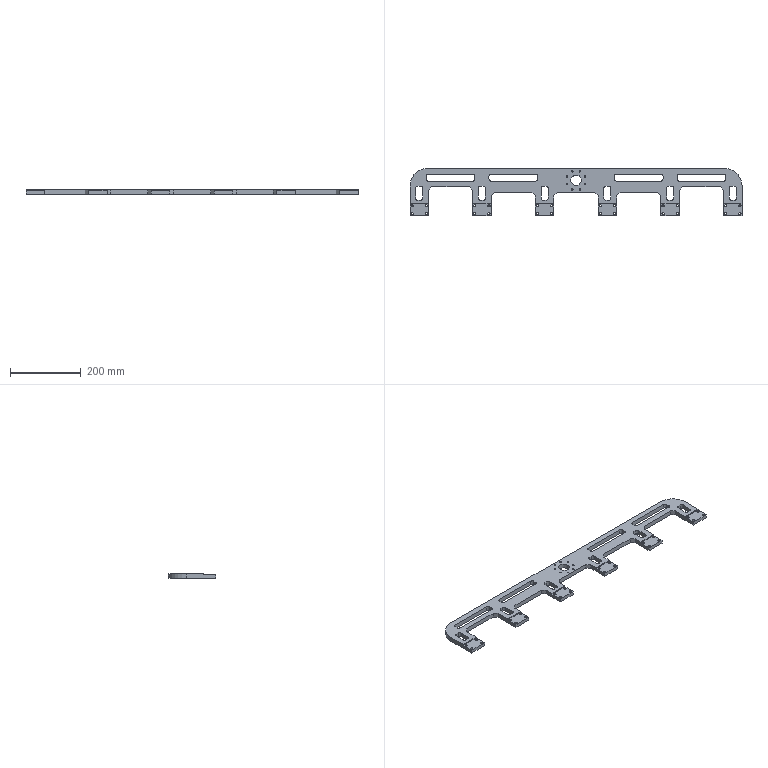Part | 1 solid | 163 faces | box 941 x 134 x 13 mm | volume 787586 mm3 | plane 88 | cylinder 75 | commonest cylinder face diameters 12 x40 6.5 x24 4.5 x8 100 x2 30 x1